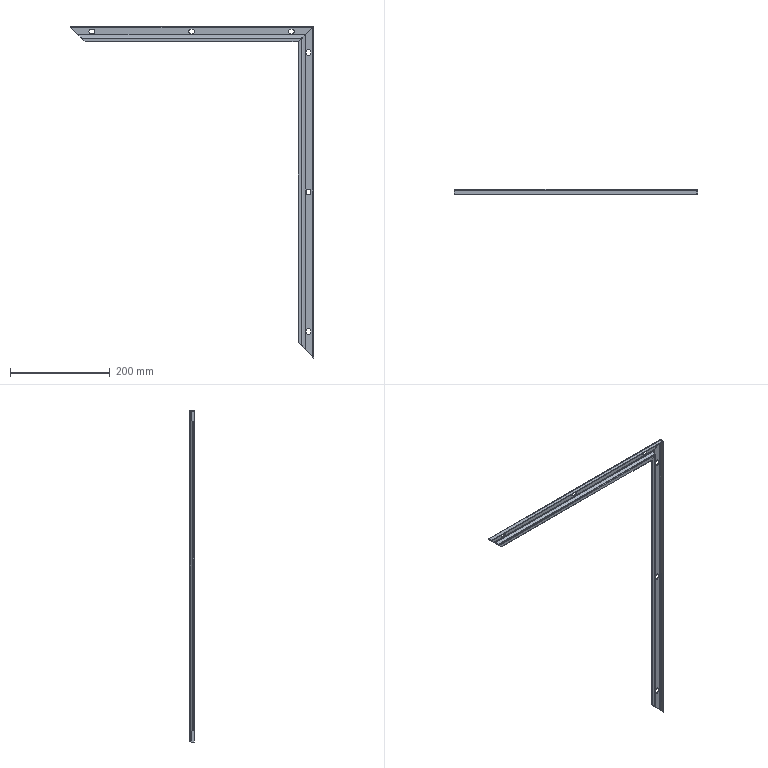Part | NX | features solid 2 | 1 solid | 87 faces | box 489.4 x 10 x 666 mm | volume 69862 mm3 | plane 46 | cylinder 29 | spline 12 | commonest cylinder face diameters 9 x15 3 x7 6 x7